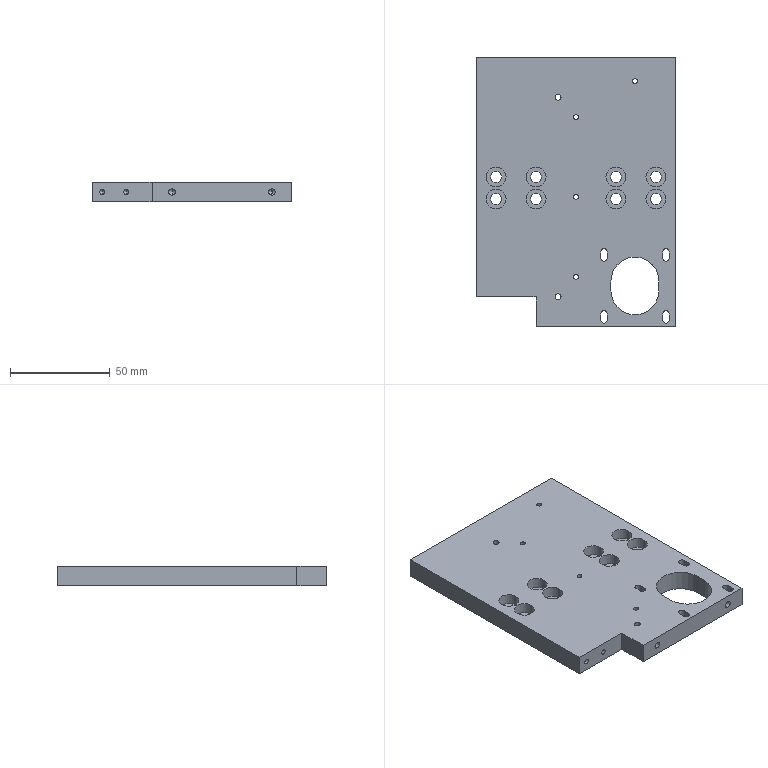Part | SolidWorks | features BaseBody 1 | 1 solid | 96 faces | box 100 x 135 x 10 mm | volume 119141 mm3 | cylinder 62 | plane 26 | cone 8 | commonest cylinder face diameters 5.5 x16 10 x16 2.459 x12 3.2 x8 3 x4 3.242 x4